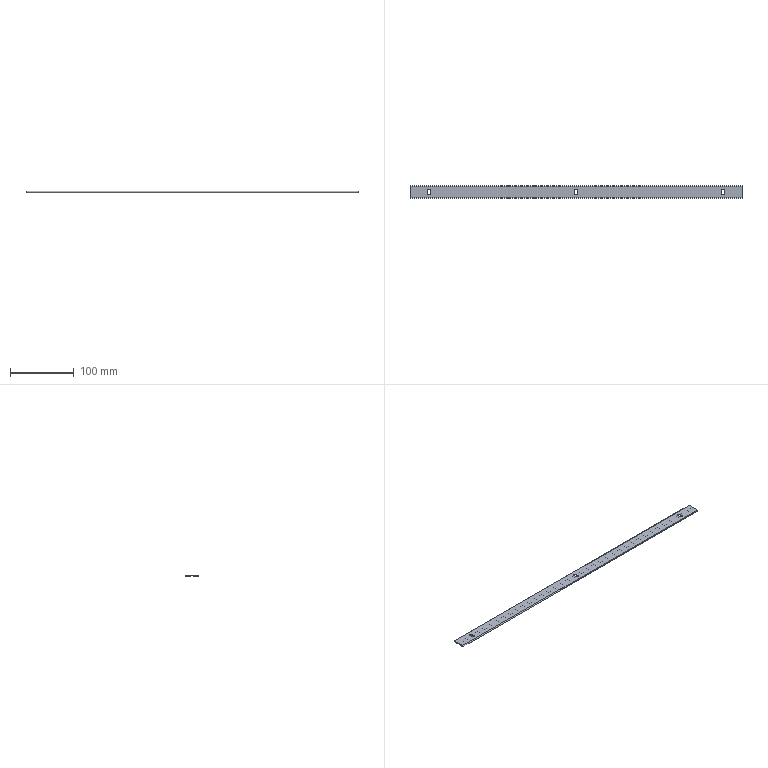Part | STEP file | HESS-408-70-15W-N-19-inner liner louver upper baffle | 1 solid | 38 faces | box 519 x 20 x 2.1 mm | volume 18114 mm3 | plane 22 | cylinder 16 | commonest cylinder face diameters 5 x6 6.5 x6 0.1 x2 2.1 x2